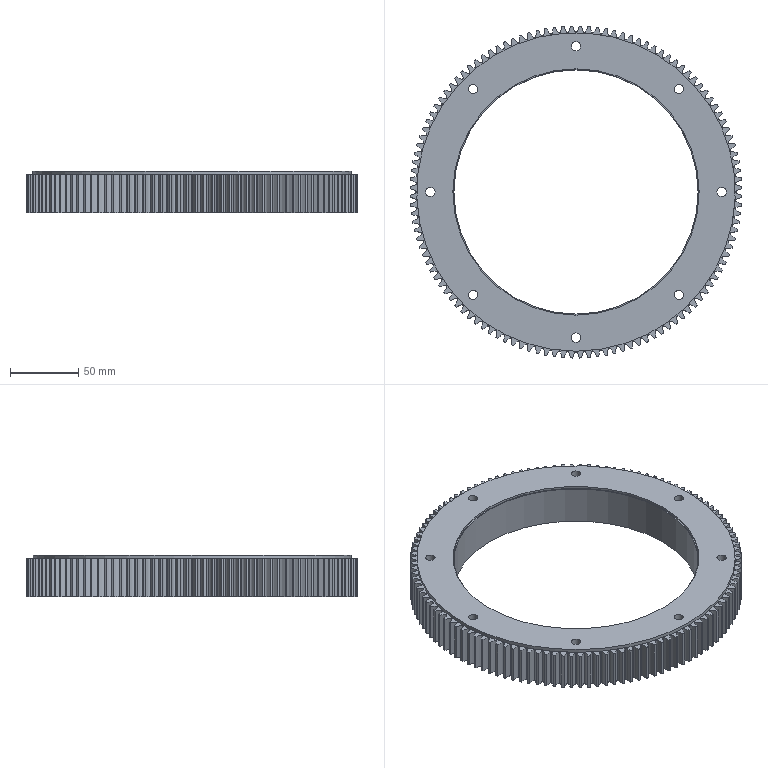Part | NX | features 5003_106_Bearing with gear 2 | 1 solid | 495 faces | box 243.954 x 243.954 x 30.5 mm | volume 587444 mm3 | spline 240 | cylinder 131 | plane 124 | commonest cylinder face diameters 244 x120 6.8 x8 179.5 x1 181 x1 234 x1